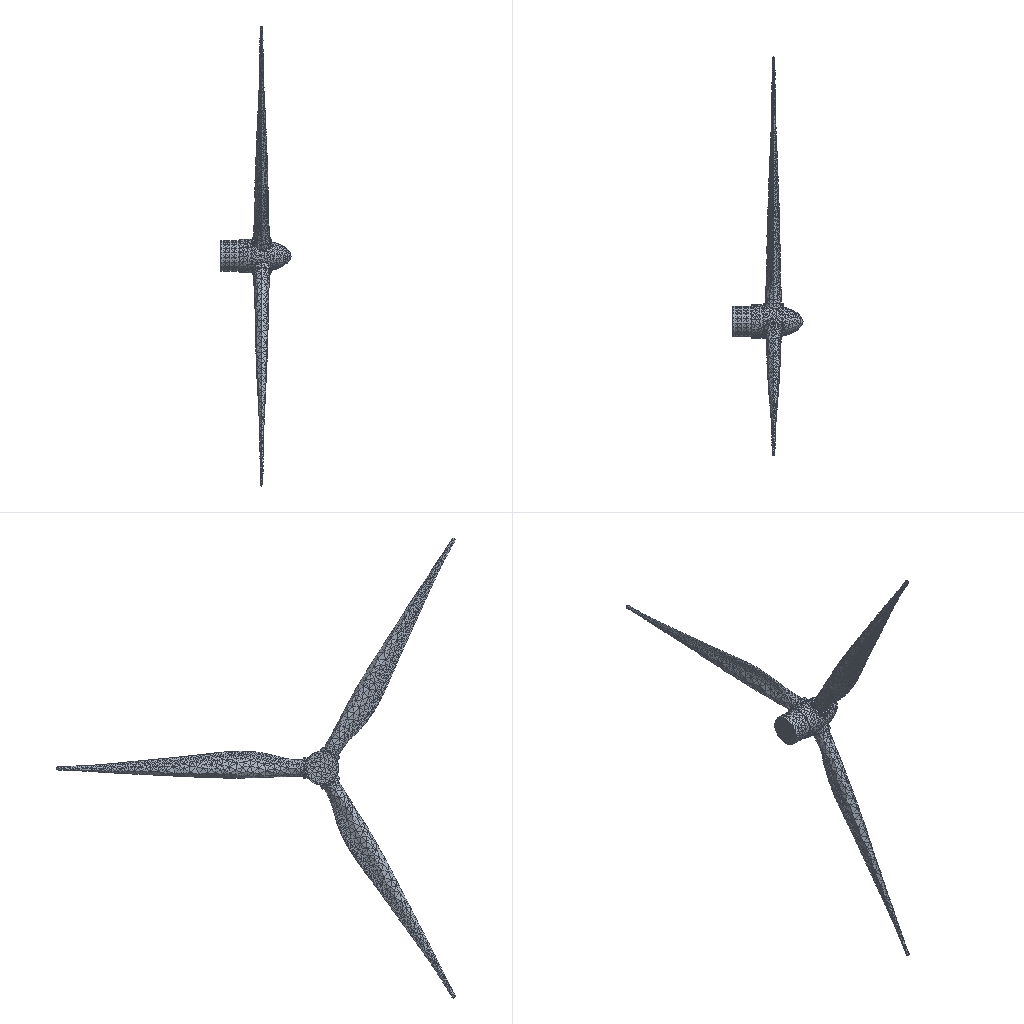Simulation study | abaqus
Set-up summary:
category,name,step,type,value,unit,region
solver,abaqus
solver,version,,,Abaqus/Standard 2020
units,not stated in the deck,,not stated
analysis,deck,,modal,modal
load_step,Step-1,Step-1,modal
load_step,requested,,,1
mesh,nodes,,,4505
mesh,elements,,,17232
element_type,C3D4,,solid,17232
load,load commands in deck,,count,0
bc,support commands in deck,,count,5
material,MATERIAL-1,,in results
material,MATERIAL-2,,in results
check,setup vs results,,match,"per instance, exact: element labels, types and connectivity; labels of the nodes the elements use; coordinates of those nodes at SINGLE_PRECISION in 1 of 1 instance(s)"
Abaqus input file, long lists of numbers shortened:
*Heading
** Job name: Job-1 Model name: Model-1
** Generated by: Abaqus/CAE 2020
*Preprint, echo=NO, model=NO, history=NO, contact=NO
**
** PARTS
**
*Part, name=Part-1
*Node
      1,   58976.211,      121000.,   57021.883
      2,   58975.773,      121000.,   56406.227
** (4503 more lines like these left out)
*Element, type=C3D4
    1, 2870, 2871, 2872, 2873
    2, 2874, 2875, 2876, 2877
** (17230 more lines like these left out)
*Nset, nset=Set-1, generate
    1,  4505,     1
*Elset, elset=Set-1, generate
     1,  17232,      1
** Section: Section-1
*Solid Section, elset=Set-1, material=Material-1
,
*End Part
**
**
** ASSEMBLY
**
*Assembly, name=Assembly
**
*Instance, name=Part-1-1, part=Part-1
*End Instance
**
*Nset, nset=Set-1, instance=Part-1-1
   43,   44,  467,  468,  469,  470,  471,  472,  473,  474,  475,  476,  477,  478,  479,  480
  481,  482,  483,  484, 1973, 1974, 1975, 1976, 1977, 1978, 1979, 1980, 1981, 1982, 1983, 1984
** (2 more lines like these left out)
*Elset, elset=Set-1, instance=Part-1-1
  1297,  3959,  3966,  4215,  4831,  6185,  6641,  7731,  8646,  8652,  8907,  9200,  9323,  9673, 10541, 11113
 11705, 12541, 12704, 12824, 13069, 13594, 13615, 13697, 14771, 14901, 14957, 15195, 15431, 15437, 15461, 15480
** (3 more lines like these left out)
*Nset, nset=Set-2, instance=Part-1-1
   43,   44,   60,   61,  467,  468,  469,  470,  471,  472,  473,  474,  475,  476,  477,  478
  479,  480,  481,  482,  483,  484,  535,  536,  537,  538,  539,  540,  541,  542,  543,  544
** (7 more lines like these left out)
*Elset, elset=Set-2, instance=Part-1-1
  1297,  3829,  3933,  3941,  3959,  3966,  4007,  4205,  4215,  4335,  4437,  4831,  4989,  5082,  5288,  5298
  5478,  5887,  5890,  6185,  6641,  6764,  7368,  7731,  7742,  7935,  8069,  8646,  8652,  8907,  8977,  9142
** (13 more lines like these left out)
*Elset, elset=_m_Surf-1_S3, internal, instance=Part-1-1
  4310,  9640, 14543, 14690, 14728, 14746, 14840, 14851, 14865, 14873, 14915, 15093, 15129, 15134, 15182, 15187
 15303, 15315, 15364, 15367, 15374
*Elset, elset=_m_Surf-1_S4, internal, instance=Part-1-1
  1961, 14891, 15137, 15144
*Elset, elset=_m_Surf-1_S1, internal, instance=Part-1-1
 14914, 15087, 15190, 15415
*Elset, elset=_m_Surf-1_S2, internal, instance=Part-1-1
  2071, 14906, 14910
*Surface, type=ELEMENT, name=m_Surf-1
_m_Surf-1_S3, S3
_m_Surf-1_S4, S4
_m_Surf-1_S2, S2
_m_Surf-1_S1, S1
*Elset, elset=_m_Surf-3_S3, internal, instance=Part-1-1
    54,   536,   695,   757,   994,  1039,  1801,  2267, 14907, 15018
*Elset, elset=_m_Surf-3_S4, internal, instance=Part-1-1
   195,   391,   627,   735, 13789
*Elset, elset=_m_Surf-3_S1, internal, instance=Part-1-1
   187,   218,   275,   632,   782,  1285, 15924, 16868
*Elset, elset=_m_Surf-3_S2, internal, instance=Part-1-1
   873,  1058,  1175,  1223,  1642,  1696,  2477, 14404, 15561
*Surface, type=ELEMENT, name=m_Surf-3
_m_Surf-3_S3, S3
_m_Surf-3_S4, S4
_m_Surf-3_S2, S2
_m_Surf-3_S1, S1
*Elset, elset=_m_Surf-5_S3, internal, instance=Part-1-1
  4358,  4747,  4849, 14422, 14452, 14462, 14469, 14569, 14749, 14754, 14758, 14765, 14768, 14778, 14780, 14783
 14787, 14789, 14800, 14808, 14824, 14834, 14889, 14925, 14978, 14992, 15226, 15262
*Elset, elset=_m_Surf-5_S2, internal, instance=Part-1-1
  1643,  2137, 15210
*Elset, elset=_m_Surf-5_S1, internal, instance=Part-1-1
 6768,
*Surface, type=ELEMENT, name=m_Surf-5
_m_Surf-5_S3, S3
_m_Surf-5_S2, S2
_m_Surf-5_S1, S1
*End Assembly
**
** MATERIALS
**
*Material, name=Material-1
*Density
1500.,
*Elastic
 1.25e+11, 0.22
*Material, name=Material-2
*Density
7800.,
*Elastic
 2.1e+11, 0.3
** ----------------------------------------------------------------
**
** STEP: Step-1
**
*Step, name=Step-1, nlgeom=NO, perturbation
*Frequency, eigensolver=Lanczos, sim, acoustic coupling=on, normalization=mass
8, , , , ,
**
** BOUNDARY CONDITIONS
**
** Name: BC-1 Type: 位移/转角
*Boundary
Set-2, 1, 1
Set-2, 2, 2
Set-2, 3, 3
Set-2, 5, 5
Set-2, 6, 6
**
** OUTPUT REQUESTS
**
*Restart, write, frequency=0
**
** FIELD OUTPUT: F-Output-1
**
*Output, field, variable=PRESELECT
*End Step
Results summary:
result,step,,partial,increments=0 time=0.0/1e-36
result,analysis,,,modal
result,last_loadstep,,,1
result,primary field,,,U